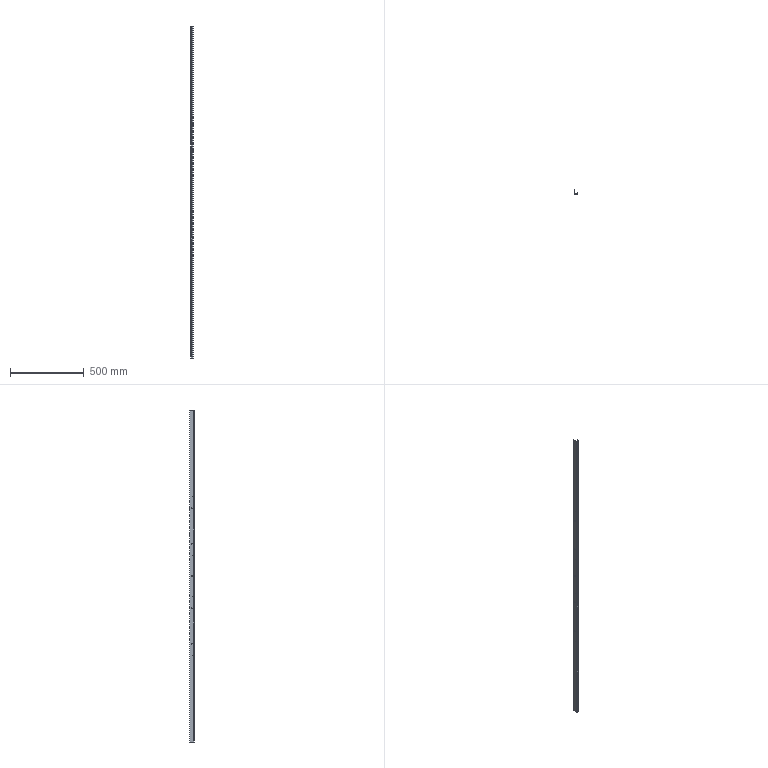Part | 1 solid | 72 faces | box 17 x 30 x 2256 mm | volume 177363 mm3 | plane 50 | cylinder 22 | commonest cylinder face diameters 6.1 x10 2 x6 5 x6